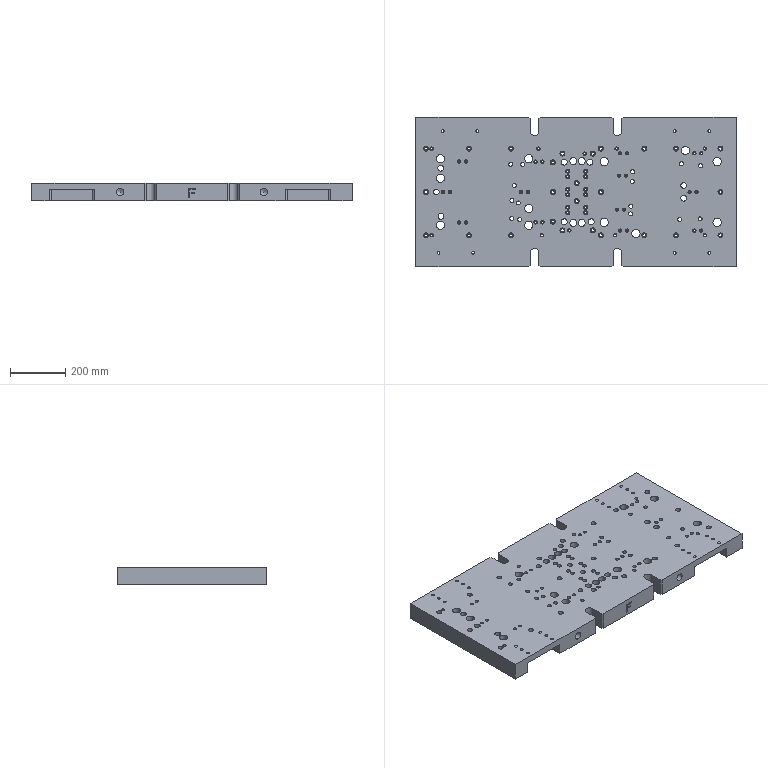Part | NX | features LIN_SOLID_COLOR 2 | 1 solid | 421 faces | box 1160 x 540 x 65 mm | volume 34876381 mm3 | cylinder 251 | plane 162 | cone 8 | commonest cylinder face diameters 12 x36 14.5 x27 7 x26 18 x26 11 x20 10.002 x16